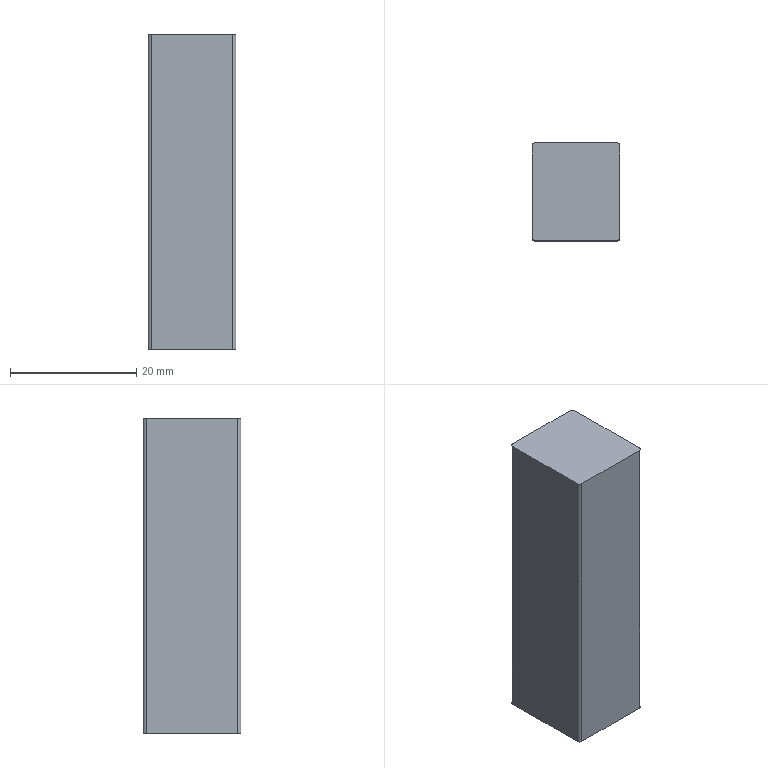Part | NX | features BREP 1 | 1 solid | 10 faces | box 13.9 x 15.498 x 50 mm | volume 10761 mm3 | plane 6 | cylinder 4 | commonest cylinder face diameters 1 x4
STEP:
#1=CARTESIAN_POINT('',(-6.45,7.749,-40.6));
#2=VERTEX_POINT('',#1);
#3=CARTESIAN_POINT('',(-6.95,7.249,-40.6));
#4=VERTEX_POINT('',#3);
#5=CARTESIAN_POINT('',(-6.45,7.249,-40.6));
#6=DIRECTION('',(0.,0.,1.));
#7=DIRECTION('',(1.,0.,0.));
#8=AXIS2_PLACEMENT_3D('',#5,#6,#7);
#9=CIRCLE('',#8,0.5);
#10=EDGE_CURVE('',#2,#4,#9,.T.);
#11=ORIENTED_EDGE('',*,*,#10,.F.);
#12=CARTESIAN_POINT('',(-6.45,7.749,-90.6));
#13=VERTEX_POINT('',#12);
#14=CARTESIAN_POINT('',(-6.45,7.749,-90.6));
#15=DIRECTION('',(0.,0.,1.));
#16=VECTOR('',#15,1000.);
#17=LINE('',#14,#16);
#18=EDGE_CURVE('',#13,#2,#17,.T.);
#19=ORIENTED_EDGE('',*,*,#18,.F.);
#20=CARTESIAN_POINT('',(-6.95,7.249,-90.6));
#21=VERTEX_POINT('',#20);
#22=CARTESIAN_POINT('',(-6.45,7.249,-90.6));
#23=DIRECTION('',(0.,0.,1.));
#24=DIRECTION('',(1.,0.,0.));
#25=AXIS2_PLACEMENT_3D('',#22,#23,#24);
#26=CIRCLE('',#25,0.5);
#27=EDGE_CURVE('',#13,#21,#26,.T.);
#28=ORIENTED_EDGE('',*,*,#27,.T.);
#29=CARTESIAN_POINT('',(-6.95,7.249,-90.6));
#30=DIRECTION('',(0.,0.,1.));
#31=VECTOR('',#30,1000.);
#32=LINE('',#29,#31);
#33=EDGE_CURVE('',#21,#4,#32,.T.);
#34=ORIENTED_EDGE('',*,*,#33,.T.);
#35=EDGE_LOOP('',(#11,#19,#28,#34));
#36=FACE_BOUND('',#35,.T.);
#37=CARTESIAN_POINT('',(-6.45,7.249,-90.6));
#38=DIRECTION('',(0.,0.,1.));
#39=DIRECTION('',(-1.,0.,0.));
#40=AXIS2_PLACEMENT_3D('',#37,#38,#39);
#41=CYLINDRICAL_SURFACE('',#40,0.5);
#42=ADVANCED_FACE('',(#36),#41,.T.);
#43=CARTESIAN_POINT('',(-6.95,-7.249,-40.6));
#44=VERTEX_POINT('',#43);
#45=CARTESIAN_POINT('',(-6.95,-7.249,-40.6));
#46=DIRECTION('',(0.,1.,0.));
#47=VECTOR('',#46,1000.);
#48=LINE('',#45,#47);
#49=EDGE_CURVE('',#44,#4,#48,.T.);
#50=ORIENTED_EDGE('',*,*,#49,.T.);
#51=ORIENTED_EDGE('',*,*,#33,.F.);
#52=CARTESIAN_POINT('',(-6.95,-7.249,-90.6));
#53=VERTEX_POINT('',#52);
#54=CARTESIAN_POINT('',(-6.95,-7.249,-90.6));
#55=DIRECTION('',(0.,1.,0.));
#56=VECTOR('',#55,1000.);
#57=LINE('',#54,#56);
#58=EDGE_CURVE('',#53,#21,#57,.T.);
#59=ORIENTED_EDGE('',*,*,#58,.F.);
#60=CARTESIAN_POINT('',(-6.95,-7.249,-90.6));
#61=DIRECTION('',(0.,0.,1.));
#62=VECTOR('',#61,1000.);
#63=LINE('',#60,#62);
#64=EDGE_CURVE('',#53,#44,#63,.T.);
#65=ORIENTED_EDGE('',*,*,#64,.T.);
#66=EDGE_LOOP('',(#50,#51,#59,#65));
#67=FACE_BOUND('',#66,.T.);
#68=CARTESIAN_POINT('',(-6.95,-7.249,-90.6));
#69=DIRECTION('',(1.,0.,0.));
#70=DIRECTION('',(0.,-1.,0.));
#71=AXIS2_PLACEMENT_3D('',#68,#69,#70);
#72=PLANE('',#71);
#73=ADVANCED_FACE('',(#67),#72,.F.);
#74=CARTESIAN_POINT('',(-6.45,-7.749,-40.6));
#75=VERTEX_POINT('',#74);
#76=CARTESIAN_POINT('',(-6.45,-7.249,-40.6));
#77=DIRECTION('',(0.,0.,1.));
#78=DIRECTION('',(1.,0.,0.));
#79=AXIS2_PLACEMENT_3D('',#76,#77,#78);
#80=CIRCLE('',#79,0.5);
#81=EDGE_CURVE('',#44,#75,#80,.T.);
#82=ORIENTED_EDGE('',*,*,#81,.F.);
#83=ORIENTED_EDGE('',*,*,#64,.F.);
#84=CARTESIAN_POINT('',(-6.45,-7.749,-90.6));
#85=VERTEX_POINT('',#84);
#86=CARTESIAN_POINT('',(-6.45,-7.249,-90.6));
#87=DIRECTION('',(0.,0.,1.));
#88=DIRECTION('',(1.,0.,0.));
#89=AXIS2_PLACEMENT_3D('',#86,#87,#88);
#90=CIRCLE('',#89,0.5);
#91=EDGE_CURVE('',#53,#85,#90,.T.);
#92=ORIENTED_EDGE('',*,*,#91,.T.);
#93=CARTESIAN_POINT('',(-6.45,-7.749,-90.6));
#94=DIRECTION('',(0.,0.,1.));
#95=VECTOR('',#94,1000.);
#96=LINE('',#93,#95);
#97=EDGE_CURVE('',#85,#75,#96,.T.);
#98=ORIENTED_EDGE('',*,*,#97,.T.);
#99=EDGE_LOOP('',(#82,#83,#92,#98));
#100=FACE_BOUND('',#99,.T.);
#101=CARTESIAN_POINT('',(-6.45,-7.249,-90.6));
#102=DIRECTION('',(0.,0.,1.));
#103=DIRECTION('',(-1.,0.,0.));
#104=AXIS2_PLACEMENT_3D('',#101,#102,#103);
#105=CYLINDRICAL_SURFACE('',#104,0.5);
#106=ADVANCED_FACE('',(#100),#105,.T.);
#107=CARTESIAN_POINT('',(6.45,-7.749,-40.6));
#108=VERTEX_POINT('',#107);
#109=CARTESIAN_POINT('',(6.45,-7.749,-40.6));
#110=DIRECTION('',(-1.,0.,0.));
#111=VECTOR('',#110,1000.);
#112=LINE('',#109,#111);
#113=EDGE_CURVE('',#108,#75,#112,.T.);
#114=ORIENTED_EDGE('',*,*,#113,.T.);
#115=ORIENTED_EDGE('',*,*,#97,.F.);
#116=CARTESIAN_POINT('',(6.45,-7.749,-90.6));
#117=VERTEX_POINT('',#116);
#118=CARTESIAN_POINT('',(6.45,-7.749,-90.6));
#119=DIRECTION('',(-1.,0.,0.));
#120=VECTOR('',#119,1000.);
#121=LINE('',#118,#120);
#122=EDGE_CURVE('',#117,#85,#121,.T.);
#123=ORIENTED_EDGE('',*,*,#122,.F.);
#124=CARTESIAN_POINT('',(6.45,-7.749,-90.6));
#125=DIRECTION('',(0.,0.,1.));
#126=VECTOR('',#125,1000.);
#127=LINE('',#124,#126);
#128=EDGE_CURVE('',#117,#108,#127,.T.);
#129=ORIENTED_EDGE('',*,*,#128,.T.);
#130=EDGE_LOOP('',(#114,#115,#123,#129));
#131=FACE_BOUND('',#130,.T.);
#132=CARTESIAN_POINT('',(6.45,-7.749,-90.6));
#133=DIRECTION('',(0.,1.,0.));
#134=DIRECTION('',(0.,0.,-1.));
#135=AXIS2_PLACEMENT_3D('',#132,#133,#134);
#136=PLANE('',#135);
#137=ADVANCED_FACE('',(#131),#136,.F.);
#138=CARTESIAN_POINT('',(6.95,-7.249,-40.6));
#139=VERTEX_POINT('',#138);
#140=CARTESIAN_POINT('',(6.45,-7.249,-40.6));
#141=DIRECTION('',(0.,0.,1.));
#142=DIRECTION('',(1.,0.,0.));
#143=AXIS2_PLACEMENT_3D('',#140,#141,#142);
#144=CIRCLE('',#143,0.5);
#145=EDGE_CURVE('',#108,#139,#144,.T.);
#146=ORIENTED_EDGE('',*,*,#145,.F.);
#147=ORIENTED_EDGE('',*,*,#128,.F.);
#148=CARTESIAN_POINT('',(6.95,-7.249,-90.6));
#149=VERTEX_POINT('',#148);
#150=CARTESIAN_POINT('',(6.45,-7.249,-90.6));
#151=DIRECTION('',(0.,0.,1.));
#152=DIRECTION('',(1.,0.,0.));
#153=AXIS2_PLACEMENT_3D('',#150,#151,#152);
#154=CIRCLE('',#153,0.5);
#155=EDGE_CURVE('',#117,#149,#154,.T.);
#156=ORIENTED_EDGE('',*,*,#155,.T.);
#157=CARTESIAN_POINT('',(6.95,-7.249,-90.6));
#158=DIRECTION('',(0.,0.,1.));
#159=VECTOR('',#158,1000.);
#160=LINE('',#157,#159);
#161=EDGE_CURVE('',#149,#139,#160,.T.);
#162=ORIENTED_EDGE('',*,*,#161,.T.);
#163=EDGE_LOOP('',(#146,#147,#156,#162));
#164=FACE_BOUND('',#163,.T.);
#165=CARTESIAN_POINT('',(6.45,-7.249,-90.6));
#166=DIRECTION('',(0.,0.,1.));
#167=DIRECTION('',(-1.,0.,0.));
#168=AXIS2_PLACEMENT_3D('',#165,#166,#167);
#169=CYLINDRICAL_SURFACE('',#168,0.5);
#170=ADVANCED_FACE('',(#164),#169,.T.);
#171=CARTESIAN_POINT('',(6.95,7.249,-40.6));
#172=VERTEX_POINT('',#171);
#173=CARTESIAN_POINT('',(6.95,7.249,-40.6));
#174=DIRECTION('',(0.,-1.,0.));
#175=VECTOR('',#174,1000.);
#176=LINE('',#173,#175);
#177=EDGE_CURVE('',#172,#139,#176,.T.);
#178=ORIENTED_EDGE('',*,*,#177,.T.);
#179=ORIENTED_EDGE('',*,*,#161,.F.);
#180=CARTESIAN_POINT('',(6.95,7.249,-90.6));
#181=VERTEX_POINT('',#180);
#182=CARTESIAN_POINT('',(6.95,7.249,-90.6));
#183=DIRECTION('',(0.,-1.,0.));
#184=VECTOR('',#183,1000.);
#185=LINE('',#182,#184);
#186=EDGE_CURVE('',#181,#149,#185,.T.);
#187=ORIENTED_EDGE('',*,*,#186,.F.);
#188=CARTESIAN_POINT('',(6.95,7.249,-90.6));
#189=DIRECTION('',(0.,0.,1.));
#190=VECTOR('',#189,1000.);
#191=LINE('',#188,#190);
#192=EDGE_CURVE('',#181,#172,#191,.T.);
#193=ORIENTED_EDGE('',*,*,#192,.T.);
#194=EDGE_LOOP('',(#178,#179,#187,#193));
#195=FACE_BOUND('',#194,.T.);
#196=CARTESIAN_POINT('',(6.95,7.249,-90.6));
#197=DIRECTION('',(-1.,0.,0.));
#198=DIRECTION('',(0.,0.,-1.));
#199=AXIS2_PLACEMENT_3D('',#196,#197,#198);
#200=PLANE('',#199);
#201=ADVANCED_FACE('',(#195),#200,.F.);
#202=CARTESIAN_POINT('',(6.45,7.749,-40.6));
#203=VERTEX_POINT('',#202);
#204=CARTESIAN_POINT('',(6.45,7.249,-40.6));
#205=DIRECTION('',(0.,0.,1.));
#206=DIRECTION('',(1.,0.,0.));
#207=AXIS2_PLACEMENT_3D('',#204,#205,#206);
#208=CIRCLE('',#207,0.5);
#209=EDGE_CURVE('',#172,#203,#208,.T.);
#210=ORIENTED_EDGE('',*,*,#209,.F.);
#211=ORIENTED_EDGE('',*,*,#192,.F.);
#212=CARTESIAN_POINT('',(6.45,7.749,-90.6));
#213=VERTEX_POINT('',#212);
#214=CARTESIAN_POINT('',(6.45,7.249,-90.6));
#215=DIRECTION('',(0.,0.,1.));
#216=DIRECTION('',(1.,0.,0.));
#217=AXIS2_PLACEMENT_3D('',#214,#215,#216);
#218=CIRCLE('',#217,0.5);
#219=EDGE_CURVE('',#181,#213,#218,.T.);
#220=ORIENTED_EDGE('',*,*,#219,.T.);
#221=CARTESIAN_POINT('',(6.45,7.749,-90.6));
#222=DIRECTION('',(0.,0.,1.));
#223=VECTOR('',#222,1000.);
#224=LINE('',#221,#223);
#225=EDGE_CURVE('',#213,#203,#224,.T.);
#226=ORIENTED_EDGE('',*,*,#225,.T.);
#227=EDGE_LOOP('',(#210,#211,#220,#226));
#228=FACE_BOUND('',#227,.T.);
#229=CARTESIAN_POINT('',(6.45,7.249,-90.6));
#230=DIRECTION('',(0.,0.,1.));
#231=DIRECTION('',(-1.,0.,0.));
#232=AXIS2_PLACEMENT_3D('',#229,#230,#231);
#233=CYLINDRICAL_SURFACE('',#232,0.5);
#234=ADVANCED_FACE('',(#228),#233,.T.);
#235=CARTESIAN_POINT('',(-6.45,7.749,-40.6));
#236=DIRECTION('',(1.,0.,0.));
#237=VECTOR('',#236,1000.);
#238=LINE('',#235,#237);
#239=EDGE_CURVE('',#2,#203,#238,.T.);
#240=ORIENTED_EDGE('',*,*,#239,.T.);
#241=ORIENTED_EDGE('',*,*,#225,.F.);
#242=CARTESIAN_POINT('',(-6.45,7.749,-90.6));
#243=DIRECTION('',(1.,0.,0.));
#244=VECTOR('',#243,1000.);
#245=LINE('',#242,#244);
#246=EDGE_CURVE('',#13,#213,#245,.T.);
#247=ORIENTED_EDGE('',*,*,#246,.F.);
#248=ORIENTED_EDGE('',*,*,#18,.T.);
#249=EDGE_LOOP('',(#240,#241,#247,#248));
#250=FACE_BOUND('',#249,.T.);
#251=CARTESIAN_POINT('',(-6.45,7.749,-90.6));
#252=DIRECTION('',(0.,-1.,0.));
#253=DIRECTION('',(0.,0.,1.));
#254=AXIS2_PLACEMENT_3D('',#251,#252,#253);
#255=PLANE('',#254);
#256=ADVANCED_FACE('',(#250),#255,.F.);
#257=ORIENTED_EDGE('',*,*,#27,.F.);
#258=ORIENTED_EDGE('',*,*,#246,.T.);
#259=ORIENTED_EDGE('',*,*,#219,.F.);
#260=ORIENTED_EDGE('',*,*,#186,.T.);
#261=ORIENTED_EDGE('',*,*,#155,.F.);
#262=ORIENTED_EDGE('',*,*,#122,.T.);
#263=ORIENTED_EDGE('',*,*,#91,.F.);
#264=ORIENTED_EDGE('',*,*,#58,.T.);
#265=EDGE_LOOP('',(#257,#258,#259,#260,#261,#262,#263,#264));
#266=FACE_BOUND('',#265,.T.);
#267=CARTESIAN_POINT('',(-6.45,7.249,-90.6));
#268=DIRECTION('',(0.,0.,1.));
#269=DIRECTION('',(-1.,0.,0.));
#270=AXIS2_PLACEMENT_3D('',#267,#268,#269);
#271=PLANE('',#270);
#272=ADVANCED_FACE('',(#266),#271,.F.);
#273=ORIENTED_EDGE('',*,*,#10,.T.);
#274=ORIENTED_EDGE('',*,*,#49,.F.);
#275=ORIENTED_EDGE('',*,*,#81,.T.);
#276=ORIENTED_EDGE('',*,*,#113,.F.);
#277=ORIENTED_EDGE('',*,*,#145,.T.);
#278=ORIENTED_EDGE('',*,*,#177,.F.);
#279=ORIENTED_EDGE('',*,*,#209,.T.);
#280=ORIENTED_EDGE('',*,*,#239,.F.);
#281=EDGE_LOOP('',(#273,#274,#275,#276,#277,#278,#279,#280));
#282=FACE_BOUND('',#281,.T.);
#283=CARTESIAN_POINT('',(-6.45,7.249,-40.6));
#284=DIRECTION('',(0.,0.,1.));
#285=DIRECTION('',(-1.,0.,0.));
#286=AXIS2_PLACEMENT_3D('',#283,#284,#285);
#287=PLANE('',#286);
#288=ADVANCED_FACE('',(#282),#287,.T.);
#289=CLOSED_SHELL('',(#42,#73,#106,#137,#170,#201,#234,#256,#272,#288));
#290=MANIFOLD_SOLID_BREP('',#289);
#291=(LENGTH_UNIT()NAMED_UNIT(*)SI_UNIT(.MILLI.,.METRE.));
#292=UNCERTAINTY_MEASURE_WITH_UNIT(LENGTH_MEASURE(0.00001),#291,'','');
#293=(NAMED_UNIT(*)PLANE_ANGLE_UNIT()SI_UNIT($,.RADIAN.));
#294=(NAMED_UNIT(*)SI_UNIT($,.STERADIAN.)SOLID_ANGLE_UNIT());
#295=(GEOMETRIC_REPRESENTATION_CONTEXT(3)GLOBAL_UNCERTAINTY_ASSIGNED_CONTEXT((#292))GLOBAL_UNIT_ASSIGNED_CONTEXT((#291,#293,#294))REPRESENTATION_CONTEXT('',''));
#296=ADVANCED_BREP_SHAPE_REPRESENTATION('',(#290),#295);